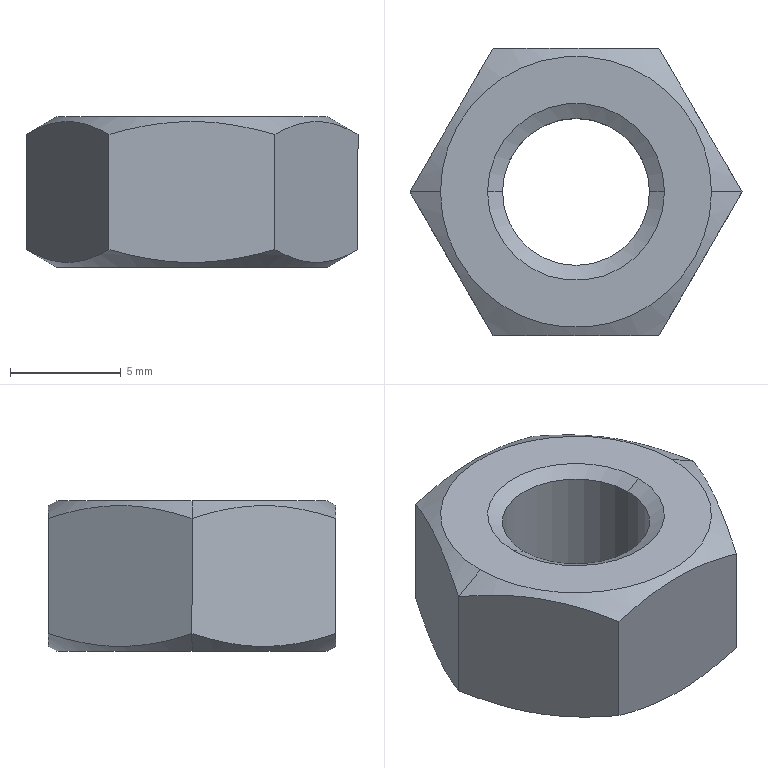Part | STEP file | hex nuts, style 1-grades ab gb_GB_FASTENER_NUT_SNAB1 M8-N | 1 solid | 18 faces | box 15.011 x 13 x 6.8 mm | volume 739.531 mm3 | cone 8 | plane 8 | cylinder 2 | commonest cylinder face diameters 6.647 x2
STEP:
#1=CARTESIAN_POINT('',(-3.324,0.,-0.3906));
#2=VERTEX_POINT('',#1);
#3=CARTESIAN_POINT('',(3.324,0.,-0.3906));
#4=VERTEX_POINT('',#3);
#5=CARTESIAN_POINT('',(0.,0.,-0.3906));
#6=DIRECTION('',(0.,0.,1.));
#7=DIRECTION('',(1.,0.,0.));
#8=AXIS2_PLACEMENT_3D('',#5,#6,#7);
#9=CIRCLE('',#8,3.324);
#10=EDGE_CURVE('',#2,#4,#9,.T.);
#11=ORIENTED_EDGE('',*,*,#10,.F.);
#12=CARTESIAN_POINT('',(-4.,0.,0.));
#13=VERTEX_POINT('',#12);
#14=CARTESIAN_POINT('',(-3.324,0.,-0.3906));
#15=DIRECTION('',(-0.866,0.,0.5));
#16=VECTOR('',#15,1000.);
#17=LINE('',#14,#16);
#18=EDGE_CURVE('',#2,#13,#17,.T.);
#19=ORIENTED_EDGE('',*,*,#18,.T.);
#20=CARTESIAN_POINT('',(4.,0.,0.));
#21=VERTEX_POINT('',#20);
#22=CARTESIAN_POINT('',(0.,0.,0.));
#23=DIRECTION('',(0.,0.,-1.));
#24=DIRECTION('',(1.,0.,0.));
#25=AXIS2_PLACEMENT_3D('',#22,#23,#24);
#26=CIRCLE('',#25,4.);
#27=EDGE_CURVE('',#21,#13,#26,.T.);
#28=ORIENTED_EDGE('',*,*,#27,.F.);
#29=CARTESIAN_POINT('',(3.324,0.,-0.3906));
#30=DIRECTION('',(0.866,0.,0.5));
#31=VECTOR('',#30,1000.);
#32=LINE('',#29,#31);
#33=EDGE_CURVE('',#4,#21,#32,.T.);
#34=ORIENTED_EDGE('',*,*,#33,.F.);
#35=EDGE_LOOP('',(#11,#19,#28,#34));
#36=FACE_OUTER_BOUND('',#35,.T.);
#37=CARTESIAN_POINT('',(0.,0.,-0.3906));
#38=DIRECTION('',(0.,0.,1.));
#39=DIRECTION('',(1.,0.,0.));
#40=AXIS2_PLACEMENT_3D('',#37,#38,#39);
#41=CONICAL_SURFACE('',#40,3.324,1.047);
#42=ADVANCED_FACE('',(#36),#41,.F.);
#43=CARTESIAN_POINT('',(3.324,0.,-6.124));
#44=VERTEX_POINT('',#43);
#45=CARTESIAN_POINT('',(-3.324,0.,-6.124));
#46=VERTEX_POINT('',#45);
#47=CARTESIAN_POINT('',(0.,0.,-6.124));
#48=DIRECTION('',(0.,0.,-1.));
#49=DIRECTION('',(1.,0.,0.));
#50=AXIS2_PLACEMENT_3D('',#47,#48,#49);
#51=CIRCLE('',#50,3.324);
#52=EDGE_CURVE('',#44,#46,#51,.T.);
#53=ORIENTED_EDGE('',*,*,#52,.F.);
#54=CARTESIAN_POINT('',(3.714,0.,-6.8));
#55=VERTEX_POINT('',#54);
#56=CARTESIAN_POINT('',(3.714,0.,-6.8));
#57=DIRECTION('',(0.5,0.,-0.866));
#58=VECTOR('',#57,1000.);
#59=LINE('',#56,#58);
#60=EDGE_CURVE('',#44,#55,#59,.T.);
#61=ORIENTED_EDGE('',*,*,#60,.T.);
#62=CARTESIAN_POINT('',(-3.714,0.,-6.8));
#63=VERTEX_POINT('',#62);
#64=CARTESIAN_POINT('',(0.,0.,-6.8));
#65=DIRECTION('',(0.,0.,1.));
#66=DIRECTION('',(1.,0.,0.));
#67=AXIS2_PLACEMENT_3D('',#64,#65,#66);
#68=CIRCLE('',#67,3.714);
#69=EDGE_CURVE('',#63,#55,#68,.T.);
#70=ORIENTED_EDGE('',*,*,#69,.F.);
#71=CARTESIAN_POINT('',(-3.714,0.,-6.8));
#72=DIRECTION('',(-0.5,0.,-0.866));
#73=VECTOR('',#72,1000.);
#74=LINE('',#71,#73);
#75=EDGE_CURVE('',#46,#63,#74,.T.);
#76=ORIENTED_EDGE('',*,*,#75,.F.);
#77=EDGE_LOOP('',(#53,#61,#70,#76));
#78=FACE_OUTER_BOUND('',#77,.T.);
#79=CARTESIAN_POINT('',(0.,0.,-6.8));
#80=DIRECTION('',(0.,0.,-1.));
#81=DIRECTION('',(-1.,0.,0.));
#82=AXIS2_PLACEMENT_3D('',#79,#80,#81);
#83=CONICAL_SURFACE('',#82,3.714,0.5236);
#84=ADVANCED_FACE('',(#78),#83,.F.);
#85=CARTESIAN_POINT('',(-6.125,0.,0.));
#86=VERTEX_POINT('',#85);
#87=CARTESIAN_POINT('',(6.125,0.,0.));
#88=VERTEX_POINT('',#87);
#89=CARTESIAN_POINT('',(0.,0.,0.));
#90=DIRECTION('',(0.,0.,-1.));
#91=DIRECTION('',(-1.,0.,0.));
#92=AXIS2_PLACEMENT_3D('',#89,#90,#91);
#93=CIRCLE('',#92,6.125);
#94=EDGE_CURVE('',#86,#88,#93,.T.);
#95=ORIENTED_EDGE('',*,*,#94,.T.);
#96=CARTESIAN_POINT('',(7.506,0.,-0.7971));
#97=VERTEX_POINT('',#96);
#98=CARTESIAN_POINT('',(6.125,0.,0.));
#99=DIRECTION('',(0.866,0.,-0.5));
#100=VECTOR('',#99,1000.);
#101=LINE('',#98,#100);
#102=EDGE_CURVE('',#88,#97,#101,.T.);
#103=ORIENTED_EDGE('',*,*,#102,.T.);
#104=CARTESIAN_POINT('',(3.753,6.5,-0.7971));
#105=VERTEX_POINT('',#104);
#106=CARTESIAN_POINT('',(7.506,0.,-0.7971));
#107=CARTESIAN_POINT('',(7.199,0.5307,-0.6202));
#108=CARTESIAN_POINT('',(6.891,1.065,-0.4744));
#109=CARTESIAN_POINT('',(6.267,2.145,-0.2724));
#110=CARTESIAN_POINT('',(5.952,2.691,-0.2169));
#111=CARTESIAN_POINT('',(5.473,3.52,-0.2163));
#112=CARTESIAN_POINT('',(5.313,3.798,-0.2299));
#113=CARTESIAN_POINT('',(4.996,4.347,-0.2828));
#114=CARTESIAN_POINT('',(4.838,4.62,-0.3221));
#115=CARTESIAN_POINT('',(4.369,5.433,-0.4738));
#116=CARTESIAN_POINT('',(4.06,5.969,-0.62));
#117=CARTESIAN_POINT('',(3.753,6.5,-0.7971));
#118=B_SPLINE_CURVE_WITH_KNOTS('',3,(#106,#107,#108,#109,#110,#111,#112,#113,#114,#115,#116,#117),.UNSPECIFIED.,.F.,.F.,(4,2,2,2,2,4),(0.000000238,0.001895,0.00379,0.004738,0.005685,0.00758),.UNSPECIFIED.);
#119=EDGE_CURVE('',#97,#105,#118,.T.);
#120=ORIENTED_EDGE('',*,*,#119,.T.);
#121=CARTESIAN_POINT('',(-3.753,6.5,-0.7971));
#122=VERTEX_POINT('',#121);
#123=CARTESIAN_POINT('',(3.753,6.5,-0.7971));
#124=CARTESIAN_POINT('',(3.146,6.5,-0.6219));
#125=CARTESIAN_POINT('',(2.532,6.5,-0.4761));
#126=CARTESIAN_POINT('',(1.278,6.5,-0.2726));
#127=CARTESIAN_POINT('',(0.6353,6.5,-0.2166));
#128=CARTESIAN_POINT('',(-0.6332,6.5,-0.2164));
#129=CARTESIAN_POINT('',(-1.263,6.5,-0.2709));
#130=CARTESIAN_POINT('',(-2.517,6.5,-0.473));
#131=CARTESIAN_POINT('',(-3.142,6.5,-0.6208));
#132=CARTESIAN_POINT('',(-3.753,6.5,-0.7971));
#133=B_SPLINE_CURVE_WITH_KNOTS('',3,(#123,#124,#125,#126,#127,#128,#129,#130,#131,#132),.UNSPECIFIED.,.F.,.F.,(4,2,2,2,4),(0.002787,0.004681,0.006575,0.008469,0.01036),.UNSPECIFIED.);
#134=EDGE_CURVE('',#105,#122,#133,.T.);
#135=ORIENTED_EDGE('',*,*,#134,.T.);
#136=CARTESIAN_POINT('',(-7.506,0.,-0.7971));
#137=VERTEX_POINT('',#136);
#138=CARTESIAN_POINT('',(-3.753,6.5,-0.7971));
#139=CARTESIAN_POINT('',(-4.059,5.969,-0.6202));
#140=CARTESIAN_POINT('',(-4.368,5.435,-0.4744));
#141=CARTESIAN_POINT('',(-4.991,4.355,-0.2724));
#142=CARTESIAN_POINT('',(-5.307,3.809,-0.2169));
#143=CARTESIAN_POINT('',(-5.785,2.98,-0.2163));
#144=CARTESIAN_POINT('',(-5.945,2.702,-0.2299));
#145=CARTESIAN_POINT('',(-6.262,2.153,-0.2828));
#146=CARTESIAN_POINT('',(-6.42,1.88,-0.3221));
#147=CARTESIAN_POINT('',(-6.889,1.067,-0.4738));
#148=CARTESIAN_POINT('',(-7.199,0.5313,-0.62));
#149=CARTESIAN_POINT('',(-7.506,0.,-0.7971));
#150=B_SPLINE_CURVE_WITH_KNOTS('',3,(#138,#139,#140,#141,#142,#143,#144,#145,#146,#147,#148,#149),.UNSPECIFIED.,.F.,.F.,(4,2,2,2,2,4),(0.000000238,0.001895,0.00379,0.004738,0.005685,0.00758),.UNSPECIFIED.);
#151=EDGE_CURVE('',#122,#137,#150,.T.);
#152=ORIENTED_EDGE('',*,*,#151,.T.);
#153=CARTESIAN_POINT('',(-6.125,0.,0.));
#154=DIRECTION('',(-0.866,0.,-0.5));
#155=VECTOR('',#154,1000.);
#156=LINE('',#153,#155);
#157=EDGE_CURVE('',#86,#137,#156,.T.);
#158=ORIENTED_EDGE('',*,*,#157,.F.);
#159=EDGE_LOOP('',(#95,#103,#120,#135,#152,#158));
#160=FACE_OUTER_BOUND('',#159,.T.);
#161=CARTESIAN_POINT('',(0.,0.,0.));
#162=DIRECTION('',(0.,0.,-1.));
#163=DIRECTION('',(-1.,0.,0.));
#164=AXIS2_PLACEMENT_3D('',#161,#162,#163);
#165=CONICAL_SURFACE('',#164,6.125,1.047);
#166=ADVANCED_FACE('',(#160),#165,.T.);
#167=CARTESIAN_POINT('',(-6.125,0.,-6.8));
#168=VERTEX_POINT('',#167);
#169=CARTESIAN_POINT('',(6.125,0.,-6.8));
#170=VERTEX_POINT('',#169);
#171=CARTESIAN_POINT('',(0.,0.,-6.8));
#172=DIRECTION('',(0.,0.,-1.));
#173=DIRECTION('',(-1.,0.,0.));
#174=AXIS2_PLACEMENT_3D('',#171,#172,#173);
#175=CIRCLE('',#174,6.125);
#176=EDGE_CURVE('',#168,#170,#175,.T.);
#177=ORIENTED_EDGE('',*,*,#176,.F.);
#178=CARTESIAN_POINT('',(-7.506,0.,-6.003));
#179=VERTEX_POINT('',#178);
#180=CARTESIAN_POINT('',(-7.506,0.,-6.003));
#181=DIRECTION('',(-0.866,0.,0.5));
#182=VECTOR('',#181,1000.);
#183=LINE('',#180,#182);
#184=EDGE_CURVE('',#168,#179,#183,.T.);
#185=ORIENTED_EDGE('',*,*,#184,.T.);
#186=CARTESIAN_POINT('',(-3.753,6.5,-6.003));
#187=VERTEX_POINT('',#186);
#188=CARTESIAN_POINT('',(-7.506,0.,-6.003));
#189=CARTESIAN_POINT('',(-7.199,0.5307,-6.18));
#190=CARTESIAN_POINT('',(-6.891,1.065,-6.326));
#191=CARTESIAN_POINT('',(-6.267,2.145,-6.528));
#192=CARTESIAN_POINT('',(-5.952,2.691,-6.583));
#193=CARTESIAN_POINT('',(-5.473,3.52,-6.584));
#194=CARTESIAN_POINT('',(-5.313,3.798,-6.57));
#195=CARTESIAN_POINT('',(-4.996,4.347,-6.517));
#196=CARTESIAN_POINT('',(-4.838,4.62,-6.478));
#197=CARTESIAN_POINT('',(-4.369,5.433,-6.326));
#198=CARTESIAN_POINT('',(-4.06,5.969,-6.18));
#199=CARTESIAN_POINT('',(-3.753,6.5,-6.003));
#200=B_SPLINE_CURVE_WITH_KNOTS('',3,(#188,#189,#190,#191,#192,#193,#194,#195,#196,#197,#198,#199),.UNSPECIFIED.,.F.,.F.,(4,2,2,2,2,4),(0.000000238,0.001895,0.00379,0.004738,0.005685,0.00758),.UNSPECIFIED.);
#201=EDGE_CURVE('',#179,#187,#200,.T.);
#202=ORIENTED_EDGE('',*,*,#201,.T.);
#203=CARTESIAN_POINT('',(3.753,6.5,-6.003));
#204=VERTEX_POINT('',#203);
#205=CARTESIAN_POINT('',(-3.753,6.5,-6.003));
#206=CARTESIAN_POINT('',(-3.142,6.5,-6.179));
#207=CARTESIAN_POINT('',(-2.517,6.5,-6.327));
#208=CARTESIAN_POINT('',(-1.263,6.5,-6.529));
#209=CARTESIAN_POINT('',(-0.6332,6.5,-6.584));
#210=CARTESIAN_POINT('',(0.6353,6.5,-6.583));
#211=CARTESIAN_POINT('',(1.278,6.5,-6.527));
#212=CARTESIAN_POINT('',(2.532,6.5,-6.324));
#213=CARTESIAN_POINT('',(3.146,6.5,-6.178));
#214=CARTESIAN_POINT('',(3.753,6.5,-6.003));
#215=B_SPLINE_CURVE_WITH_KNOTS('',3,(#205,#206,#207,#208,#209,#210,#211,#212,#213,#214),.UNSPECIFIED.,.F.,.F.,(4,2,2,2,4),(0.006662,0.008561,0.01046,0.01236,0.01426),.UNSPECIFIED.);
#216=EDGE_CURVE('',#187,#204,#215,.T.);
#217=ORIENTED_EDGE('',*,*,#216,.T.);
#218=CARTESIAN_POINT('',(7.506,0.,-6.003));
#219=VERTEX_POINT('',#218);
#220=CARTESIAN_POINT('',(3.753,6.5,-6.003));
#221=CARTESIAN_POINT('',(4.059,5.969,-6.18));
#222=CARTESIAN_POINT('',(4.368,5.435,-6.326));
#223=CARTESIAN_POINT('',(4.991,4.355,-6.528));
#224=CARTESIAN_POINT('',(5.307,3.809,-6.583));
#225=CARTESIAN_POINT('',(5.785,2.98,-6.584));
#226=CARTESIAN_POINT('',(5.945,2.702,-6.57));
#227=CARTESIAN_POINT('',(6.262,2.153,-6.517));
#228=CARTESIAN_POINT('',(6.42,1.88,-6.478));
#229=CARTESIAN_POINT('',(6.889,1.067,-6.326));
#230=CARTESIAN_POINT('',(7.199,0.5313,-6.18));
#231=CARTESIAN_POINT('',(7.506,0.,-6.003));
#232=B_SPLINE_CURVE_WITH_KNOTS('',3,(#220,#221,#222,#223,#224,#225,#226,#227,#228,#229,#230,#231),.UNSPECIFIED.,.F.,.F.,(4,2,2,2,2,4),(0.000000238,0.001895,0.00379,0.004738,0.005685,0.00758),.UNSPECIFIED.);
#233=EDGE_CURVE('',#204,#219,#232,.T.);
#234=ORIENTED_EDGE('',*,*,#233,.T.);
#235=CARTESIAN_POINT('',(7.506,0.,-6.003));
#236=DIRECTION('',(0.866,0.,0.5));
#237=VECTOR('',#236,1000.);
#238=LINE('',#235,#237);
#239=EDGE_CURVE('',#170,#219,#238,.T.);
#240=ORIENTED_EDGE('',*,*,#239,.F.);
#241=EDGE_LOOP('',(#177,#185,#202,#217,#234,#240));
#242=FACE_OUTER_BOUND('',#241,.T.);
#243=CARTESIAN_POINT('',(0.,0.,-6.003));
#244=DIRECTION('',(0.,0.,1.));
#245=DIRECTION('',(1.,0.,0.));
#246=AXIS2_PLACEMENT_3D('',#243,#244,#245);
#247=CONICAL_SURFACE('',#246,7.506,1.047);
#248=ADVANCED_FACE('',(#242),#247,.T.);
#249=ORIENTED_EDGE('',*,*,#52,.T.);
#250=CARTESIAN_POINT('',(-3.324,0.,-6.8));
#251=DIRECTION('',(0.,0.,1.));
#252=VECTOR('',#251,1000.);
#253=LINE('',#250,#252);
#254=EDGE_CURVE('',#46,#2,#253,.T.);
#255=ORIENTED_EDGE('',*,*,#254,.T.);
#256=ORIENTED_EDGE('',*,*,#10,.T.);
#257=CARTESIAN_POINT('',(3.324,0.,-6.8));
#258=DIRECTION('',(0.,0.,1.));
#259=VECTOR('',#258,1000.);
#260=LINE('',#257,#259);
#261=EDGE_CURVE('',#44,#4,#260,.T.);
#262=ORIENTED_EDGE('',*,*,#261,.F.);
#263=EDGE_LOOP('',(#249,#255,#256,#262));
#264=FACE_OUTER_BOUND('',#263,.T.);
#265=CARTESIAN_POINT('',(0.,0.,-6.8));
#266=DIRECTION('',(0.,0.,1.));
#267=DIRECTION('',(1.,0.,0.));
#268=AXIS2_PLACEMENT_3D('',#265,#266,#267);
#269=CYLINDRICAL_SURFACE('',#268,3.324);
#270=ADVANCED_FACE('',(#264),#269,.F.);
#271=CARTESIAN_POINT('',(3.753,-6.5,-0.7971));
#272=VERTEX_POINT('',#271);
#273=CARTESIAN_POINT('',(3.753,-6.5,-0.7971));
#274=CARTESIAN_POINT('',(4.059,-5.969,-0.6202));
#275=CARTESIAN_POINT('',(4.368,-5.435,-0.4744));
#276=CARTESIAN_POINT('',(4.991,-4.355,-0.2724));
#277=CARTESIAN_POINT('',(5.307,-3.809,-0.2169));
#278=CARTESIAN_POINT('',(5.785,-2.98,-0.2163));
#279=CARTESIAN_POINT('',(5.945,-2.702,-0.2299));
#280=CARTESIAN_POINT('',(6.262,-2.153,-0.2828));
#281=CARTESIAN_POINT('',(6.42,-1.88,-0.3221));
#282=CARTESIAN_POINT('',(6.889,-1.067,-0.4738));
#283=CARTESIAN_POINT('',(7.199,-0.5313,-0.62));
#284=CARTESIAN_POINT('',(7.506,0.,-0.7971));
#285=B_SPLINE_CURVE_WITH_KNOTS('',3,(#273,#274,#275,#276,#277,#278,#279,#280,#281,#282,#283,#284),.UNSPECIFIED.,.F.,.F.,(4,2,2,2,2,4),(0.000000238,0.001895,0.00379,0.004738,0.005685,0.00758),.UNSPECIFIED.);
#286=EDGE_CURVE('',#272,#97,#285,.T.);
#287=ORIENTED_EDGE('',*,*,#286,.F.);
#288=CARTESIAN_POINT('',(3.753,-6.5,-6.003));
#289=VERTEX_POINT('',#288);
#290=CARTESIAN_POINT('',(3.753,-6.5,-6.8));
#291=DIRECTION('',(0.,0.,1.));
#292=VECTOR('',#291,1000.);
#293=LINE('',#290,#292);
#294=EDGE_CURVE('',#289,#272,#293,.T.);
#295=ORIENTED_EDGE('',*,*,#294,.F.);
#296=CARTESIAN_POINT('',(7.506,0.,-6.003));
#297=CARTESIAN_POINT('',(7.199,-0.5307,-6.18));
#298=CARTESIAN_POINT('',(6.891,-1.065,-6.326));
#299=CARTESIAN_POINT('',(6.267,-2.145,-6.528));
#300=CARTESIAN_POINT('',(5.952,-2.691,-6.583));
#301=CARTESIAN_POINT('',(5.473,-3.52,-6.584));
#302=CARTESIAN_POINT('',(5.313,-3.798,-6.57));
#303=CARTESIAN_POINT('',(4.996,-4.347,-6.517));
#304=CARTESIAN_POINT('',(4.838,-4.62,-6.478));
#305=CARTESIAN_POINT('',(4.369,-5.433,-6.326));
#306=CARTESIAN_POINT('',(4.06,-5.969,-6.18));
#307=CARTESIAN_POINT('',(3.753,-6.5,-6.003));
#308=B_SPLINE_CURVE_WITH_KNOTS('',3,(#296,#297,#298,#299,#300,#301,#302,#303,#304,#305,#306,#307),.UNSPECIFIED.,.F.,.F.,(4,2,2,2,2,4),(0.000000238,0.001895,0.00379,0.004738,0.005685,0.00758),.UNSPECIFIED.);
#309=EDGE_CURVE('',#219,#289,#308,.T.);
#310=ORIENTED_EDGE('',*,*,#309,.F.);
#311=CARTESIAN_POINT('',(7.506,0.,-6.8));
#312=DIRECTION('',(0.,0.,1.));
#313=VECTOR('',#312,1000.);
#314=LINE('',#311,#313);
#315=EDGE_CURVE('',#219,#97,#314,.T.);
#316=ORIENTED_EDGE('',*,*,#315,.T.);
#317=EDGE_LOOP('',(#287,#295,#310,#316));
#318=FACE_OUTER_BOUND('',#317,.T.);
#319=CARTESIAN_POINT('',(3.753,-6.5,-6.8));
#320=DIRECTION('',(0.866,-0.5,0.));
#321=DIRECTION('',(0.5,0.866,0.));
#322=AXIS2_PLACEMENT_3D('',#319,#320,#321);
#323=PLANE('',#322);
#324=ADVANCED_FACE('',(#318),#323,.T.);
#325=CARTESIAN_POINT('',(-3.753,-6.5,-0.7971));
#326=VERTEX_POINT('',#325);
#327=CARTESIAN_POINT('',(-3.753,-6.5,-0.7971));
#328=CARTESIAN_POINT('',(-3.142,-6.5,-0.6208));
#329=CARTESIAN_POINT('',(-2.517,-6.5,-0.473));
#330=CARTESIAN_POINT('',(-1.263,-6.5,-0.2709));
#331=CARTESIAN_POINT('',(-0.6332,-6.5,-0.2164));
#332=CARTESIAN_POINT('',(0.6353,-6.5,-0.2166));
#333=CARTESIAN_POINT('',(1.278,-6.5,-0.2726));
#334=CARTESIAN_POINT('',(2.532,-6.5,-0.4761));
#335=CARTESIAN_POINT('',(3.146,-6.5,-0.6219));
#336=CARTESIAN_POINT('',(3.753,-6.5,-0.7971));
#337=B_SPLINE_CURVE_WITH_KNOTS('',3,(#327,#328,#329,#330,#331,#332,#333,#334,#335,#336),.UNSPECIFIED.,.F.,.F.,(4,2,2,2,4),(0.006662,0.008561,0.01046,0.01236,0.01426),.UNSPECIFIED.);
#338=EDGE_CURVE('',#326,#272,#337,.T.);
#339=ORIENTED_EDGE('',*,*,#338,.F.);
#340=CARTESIAN_POINT('',(-3.753,-6.5,-6.003));
#341=VERTEX_POINT('',#340);
#342=CARTESIAN_POINT('',(-3.753,-6.5,-6.8));
#343=DIRECTION('',(0.,0.,1.));
#344=VECTOR('',#343,1000.);
#345=LINE('',#342,#344);
#346=EDGE_CURVE('',#341,#326,#345,.T.);
#347=ORIENTED_EDGE('',*,*,#346,.F.);
#348=CARTESIAN_POINT('',(3.753,-6.5,-6.003));
#349=CARTESIAN_POINT('',(3.146,-6.5,-6.178));
#350=CARTESIAN_POINT('',(2.532,-6.5,-6.324));
#351=CARTESIAN_POINT('',(1.278,-6.5,-6.527));
#352=CARTESIAN_POINT('',(0.6353,-6.5,-6.583));
#353=CARTESIAN_POINT('',(-0.6332,-6.5,-6.584));
#354=CARTESIAN_POINT('',(-1.263,-6.5,-6.529));
#355=CARTESIAN_POINT('',(-2.517,-6.5,-6.327));
#356=CARTESIAN_POINT('',(-3.142,-6.5,-6.179));
#357=CARTESIAN_POINT('',(-3.753,-6.5,-6.003));
#358=B_SPLINE_CURVE_WITH_KNOTS('',3,(#348,#349,#350,#351,#352,#353,#354,#355,#356,#357),.UNSPECIFIED.,.F.,.F.,(4,2,2,2,4),(0.002787,0.004681,0.006575,0.008469,0.01036),.UNSPECIFIED.);
#359=EDGE_CURVE('',#289,#341,#358,.T.);
#360=ORIENTED_EDGE('',*,*,#359,.F.);
#361=ORIENTED_EDGE('',*,*,#294,.T.);
#362=EDGE_LOOP('',(#339,#347,#360,#361));
#363=FACE_OUTER_BOUND('',#362,.T.);
#364=CARTESIAN_POINT('',(-3.753,-6.5,-6.8));
#365=DIRECTION('',(0.,-1.,0.));
#366=DIRECTION('',(0.,0.,-1.));
#367=AXIS2_PLACEMENT_3D('',#364,#365,#366);
#368=PLANE('',#367);
#369=ADVANCED_FACE('',(#363),#368,.T.);
#370=CARTESIAN_POINT('',(-7.506,0.,-0.7971));
#371=CARTESIAN_POINT('',(-7.199,-0.5307,-0.6202));
#372=CARTESIAN_POINT('',(-6.891,-1.065,-0.4744));
#373=CARTESIAN_POINT('',(-6.267,-2.145,-0.2724));
#374=CARTESIAN_POINT('',(-5.952,-2.691,-0.2169));
#375=CARTESIAN_POINT('',(-5.473,-3.52,-0.2163));
#376=CARTESIAN_POINT('',(-5.313,-3.798,-0.2299));
#377=CARTESIAN_POINT('',(-4.996,-4.347,-0.2828));
#378=CARTESIAN_POINT('',(-4.838,-4.62,-0.3221));
#379=CARTESIAN_POINT('',(-4.369,-5.433,-0.4738));
#380=CARTESIAN_POINT('',(-4.06,-5.969,-0.62));
#381=CARTESIAN_POINT('',(-3.753,-6.5,-0.7971));
#382=B_SPLINE_CURVE_WITH_KNOTS('',3,(#370,#371,#372,#373,#374,#375,#376,#377,#378,#379,#380,#381),.UNSPECIFIED.,.F.,.F.,(4,2,2,2,2,4),(0.000000238,0.001895,0.00379,0.004738,0.005685,0.00758),.UNSPECIFIED.);
#383=EDGE_CURVE('',#137,#326,#382,.T.);
#384=ORIENTED_EDGE('',*,*,#383,.F.);
#385=CARTESIAN_POINT('',(-7.506,0.,-6.8));
#386=DIRECTION('',(0.,0.,1.));
#387=VECTOR('',#386,1000.);
#388=LINE('',#385,#387);
#389=EDGE_CURVE('',#179,#137,#388,.T.);
#390=ORIENTED_EDGE('',*,*,#389,.F.);
#391=CARTESIAN_POINT('',(-3.753,-6.5,-6.003));
#392=CARTESIAN_POINT('',(-4.059,-5.969,-6.18));
#393=CARTESIAN_POINT('',(-4.368,-5.435,-6.326));
#394=CARTESIAN_POINT('',(-4.991,-4.355,-6.528));
#395=CARTESIAN_POINT('',(-5.307,-3.809,-6.583));
#396=CARTESIAN_POINT('',(-5.785,-2.98,-6.584));
#397=CARTESIAN_POINT('',(-5.945,-2.702,-6.57));
#398=CARTESIAN_POINT('',(-6.262,-2.153,-6.517));
#399=CARTESIAN_POINT('',(-6.42,-1.88,-6.478));
#400=CARTESIAN_POINT('',(-6.889,-1.067,-6.326));
#401=CARTESIAN_POINT('',(-7.199,-0.5313,-6.18));
#402=CARTESIAN_POINT('',(-7.506,0.,-6.003));
#403=B_SPLINE_CURVE_WITH_KNOTS('',3,(#391,#392,#393,#394,#395,#396,#397,#398,#399,#400,#401,#402),.UNSPECIFIED.,.F.,.F.,(4,2,2,2,2,4),(0.000000238,0.001895,0.00379,0.004738,0.005685,0.00758),.UNSPECIFIED.);
#404=EDGE_CURVE('',#341,#179,#403,.T.);
#405=ORIENTED_EDGE('',*,*,#404,.F.);
#406=ORIENTED_EDGE('',*,*,#346,.T.);
#407=EDGE_LOOP('',(#384,#390,#405,#406));
#408=FACE_OUTER_BOUND('',#407,.T.);
#409=CARTESIAN_POINT('',(-7.506,0.,-6.8));
#410=DIRECTION('',(-0.866,-0.5,0.));
#411=DIRECTION('',(0.5,-0.866,0.));
#412=AXIS2_PLACEMENT_3D('',#409,#410,#411);
#413=PLANE('',#412);
#414=ADVANCED_FACE('',(#408),#413,.T.);
#415=ORIENTED_EDGE('',*,*,#151,.F.);
#416=CARTESIAN_POINT('',(-3.753,6.5,-6.8));
#417=DIRECTION('',(0.,0.,1.));
#418=VECTOR('',#417,1000.);
#419=LINE('',#416,#418);
#420=EDGE_CURVE('',#187,#122,#419,.T.);
#421=ORIENTED_EDGE('',*,*,#420,.F.);
#422=ORIENTED_EDGE('',*,*,#201,.F.);
#423=ORIENTED_EDGE('',*,*,#389,.T.);
#424=EDGE_LOOP('',(#415,#421,#422,#423));
#425=FACE_OUTER_BOUND('',#424,.T.);
#426=CARTESIAN_POINT('',(-3.753,6.5,-6.8));
#427=DIRECTION('',(-0.866,0.5,0.));
#428=DIRECTION('',(-0.5,-0.866,0.));
#429=AXIS2_PLACEMENT_3D('',#426,#427,#428);
#430=PLANE('',#429);
#431=ADVANCED_FACE('',(#425),#430,.T.);
#432=ORIENTED_EDGE('',*,*,#134,.F.);
#433=CARTESIAN_POINT('',(3.753,6.5,-6.8));
#434=DIRECTION('',(0.,0.,1.));
#435=VECTOR('',#434,1000.);
#436=LINE('',#433,#435);
#437=EDGE_CURVE('',#204,#105,#436,.T.);
#438=ORIENTED_EDGE('',*,*,#437,.F.);
#439=ORIENTED_EDGE('',*,*,#216,.F.);
#440=ORIENTED_EDGE('',*,*,#420,.T.);
#441=EDGE_LOOP('',(#432,#438,#439,#440));
#442=FACE_OUTER_BOUND('',#441,.T.);
#443=CARTESIAN_POINT('',(3.753,6.5,-6.8));
#444=DIRECTION('',(0.,1.,0.));
#445=DIRECTION('',(0.,0.,1.));
#446=AXIS2_PLACEMENT_3D('',#443,#444,#445);
#447=PLANE('',#446);
#448=ADVANCED_FACE('',(#442),#447,.T.);
#449=ORIENTED_EDGE('',*,*,#119,.F.);
#450=ORIENTED_EDGE('',*,*,#315,.F.);
#451=ORIENTED_EDGE('',*,*,#233,.F.);
#452=ORIENTED_EDGE('',*,*,#437,.T.);
#453=EDGE_LOOP('',(#449,#450,#451,#452));
#454=FACE_OUTER_BOUND('',#453,.T.);
#455=CARTESIAN_POINT('',(7.506,0.,-6.8));
#456=DIRECTION('',(0.866,0.5,0.));
#457=DIRECTION('',(-0.5,0.866,0.));
#458=AXIS2_PLACEMENT_3D('',#455,#456,#457);
#459=PLANE('',#458);
#460=ADVANCED_FACE('',(#454),#459,.T.);
#461=ORIENTED_EDGE('',*,*,#69,.T.);
#462=CARTESIAN_POINT('',(0.,0.,-6.8));
#463=DIRECTION('',(0.,0.,1.));
#464=DIRECTION('',(1.,0.,0.));
#465=AXIS2_PLACEMENT_3D('',#462,#463,#464);
#466=CIRCLE('',#465,3.714);
#467=EDGE_CURVE('',#55,#63,#466,.T.);
#468=ORIENTED_EDGE('',*,*,#467,.T.);
#469=EDGE_LOOP('',(#461,#468));
#470=FACE_BOUND('',#469,.T.);
#471=CARTESIAN_POINT('',(0.,0.,-6.8));
#472=DIRECTION('',(0.,0.,-1.));
#473=DIRECTION('',(-1.,0.,0.));
#474=AXIS2_PLACEMENT_3D('',#471,#472,#473);
#475=CIRCLE('',#474,6.125);
#476=EDGE_CURVE('',#170,#168,#475,.T.);
#477=ORIENTED_EDGE('',*,*,#476,.T.);
#478=ORIENTED_EDGE('',*,*,#176,.T.);
#479=EDGE_LOOP('',(#477,#478));
#480=FACE_OUTER_BOUND('',#479,.T.);
#481=CARTESIAN_POINT('',(7.506,0.,-6.8));
#482=DIRECTION('',(0.,0.,1.));
#483=DIRECTION('',(1.,0.,0.));
#484=AXIS2_PLACEMENT_3D('',#481,#482,#483);
#485=PLANE('',#484);
#486=ADVANCED_FACE('',(#470,#480),#485,.F.);
#487=ORIENTED_EDGE('',*,*,#27,.T.);
#488=CARTESIAN_POINT('',(0.,0.,0.));
#489=DIRECTION('',(0.,0.,-1.));
#490=DIRECTION('',(1.,0.,0.));
#491=AXIS2_PLACEMENT_3D('',#488,#489,#490);
#492=CIRCLE('',#491,4.);
#493=EDGE_CURVE('',#13,#21,#492,.T.);
#494=ORIENTED_EDGE('',*,*,#493,.T.);
#495=EDGE_LOOP('',(#487,#494));
#496=FACE_BOUND('',#495,.T.);
#497=ORIENTED_EDGE('',*,*,#94,.F.);
#498=CARTESIAN_POINT('',(0.,0.,0.));
#499=DIRECTION('',(0.,0.,-1.));
#500=DIRECTION('',(-1.,0.,0.));
#501=AXIS2_PLACEMENT_3D('',#498,#499,#500);
#502=CIRCLE('',#501,6.125);
#503=EDGE_CURVE('',#88,#86,#502,.T.);
#504=ORIENTED_EDGE('',*,*,#503,.F.);
#505=EDGE_LOOP('',(#497,#504));
#506=FACE_OUTER_BOUND('',#505,.T.);
#507=CARTESIAN_POINT('',(7.506,0.,0.));
#508=DIRECTION('',(0.,0.,1.));
#509=DIRECTION('',(1.,0.,0.));
#510=AXIS2_PLACEMENT_3D('',#507,#508,#509);
#511=PLANE('',#510);
#512=ADVANCED_FACE('',(#496,#506),#511,.T.);
#513=ORIENTED_EDGE('',*,*,#254,.F.);
#514=CARTESIAN_POINT('',(0.,0.,-6.124));
#515=DIRECTION('',(0.,0.,-1.));
#516=DIRECTION('',(1.,0.,0.));
#517=AXIS2_PLACEMENT_3D('',#514,#515,#516);
#518=CIRCLE('',#517,3.324);
#519=EDGE_CURVE('',#46,#44,#518,.T.);
#520=ORIENTED_EDGE('',*,*,#519,.T.);
#521=ORIENTED_EDGE('',*,*,#261,.T.);
#522=CARTESIAN_POINT('',(0.,0.,-0.3906));
#523=DIRECTION('',(0.,0.,1.));
#524=DIRECTION('',(1.,0.,0.));
#525=AXIS2_PLACEMENT_3D('',#522,#523,#524);
#526=CIRCLE('',#525,3.324);
#527=EDGE_CURVE('',#4,#2,#526,.T.);
#528=ORIENTED_EDGE('',*,*,#527,.T.);
#529=EDGE_LOOP('',(#513,#520,#521,#528));
#530=FACE_OUTER_BOUND('',#529,.T.);
#531=CARTESIAN_POINT('',(0.,0.,-6.8));
#532=DIRECTION('',(0.,0.,1.));
#533=DIRECTION('',(1.,0.,0.));
#534=AXIS2_PLACEMENT_3D('',#531,#532,#533);
#535=CYLINDRICAL_SURFACE('',#534,3.324);
#536=ADVANCED_FACE('',(#530),#535,.F.);
#537=ORIENTED_EDGE('',*,*,#184,.F.);
#538=ORIENTED_EDGE('',*,*,#476,.F.);
#539=ORIENTED_EDGE('',*,*,#239,.T.);
#540=ORIENTED_EDGE('',*,*,#309,.T.);
#541=ORIENTED_EDGE('',*,*,#359,.T.);
#542=ORIENTED_EDGE('',*,*,#404,.T.);
#543=EDGE_LOOP('',(#537,#538,#539,#540,#541,#542));
#544=FACE_OUTER_BOUND('',#543,.T.);
#545=CARTESIAN_POINT('',(0.,0.,-6.003));
#546=DIRECTION('',(0.,0.,1.));
#547=DIRECTION('',(1.,0.,0.));
#548=AXIS2_PLACEMENT_3D('',#545,#546,#547);
#549=CONICAL_SURFACE('',#548,7.506,1.047);
#550=ADVANCED_FACE('',(#544),#549,.T.);
#551=ORIENTED_EDGE('',*,*,#102,.F.);
#552=ORIENTED_EDGE('',*,*,#503,.T.);
#553=ORIENTED_EDGE('',*,*,#157,.T.);
#554=ORIENTED_EDGE('',*,*,#383,.T.);
#555=ORIENTED_EDGE('',*,*,#338,.T.);
#556=ORIENTED_EDGE('',*,*,#286,.T.);
#557=EDGE_LOOP('',(#551,#552,#553,#554,#555,#556));
#558=FACE_OUTER_BOUND('',#557,.T.);
#559=CARTESIAN_POINT('',(0.,0.,0.));
#560=DIRECTION('',(0.,0.,-1.));
#561=DIRECTION('',(-1.,0.,0.));
#562=AXIS2_PLACEMENT_3D('',#559,#560,#561);
#563=CONICAL_SURFACE('',#562,6.125,1.047);
#564=ADVANCED_FACE('',(#558),#563,.T.);
#565=ORIENTED_EDGE('',*,*,#60,.F.);
#566=ORIENTED_EDGE('',*,*,#519,.F.);
#567=ORIENTED_EDGE('',*,*,#75,.T.);
#568=ORIENTED_EDGE('',*,*,#467,.F.);
#569=EDGE_LOOP('',(#565,#566,#567,#568));
#570=FACE_OUTER_BOUND('',#569,.T.);
#571=CARTESIAN_POINT('',(0.,0.,-6.8));
#572=DIRECTION('',(0.,0.,-1.));
#573=DIRECTION('',(-1.,0.,0.));
#574=AXIS2_PLACEMENT_3D('',#571,#572,#573);
#575=CONICAL_SURFACE('',#574,3.714,0.5236);
#576=ADVANCED_FACE('',(#570),#575,.F.);
#577=ORIENTED_EDGE('',*,*,#18,.F.);
#578=ORIENTED_EDGE('',*,*,#527,.F.);
#579=ORIENTED_EDGE('',*,*,#33,.T.);
#580=ORIENTED_EDGE('',*,*,#493,.F.);
#581=EDGE_LOOP('',(#577,#578,#579,#580));
#582=FACE_OUTER_BOUND('',#581,.T.);
#583=CARTESIAN_POINT('',(0.,0.,-0.3906));
#584=DIRECTION('',(0.,0.,1.));
#585=DIRECTION('',(1.,0.,0.));
#586=AXIS2_PLACEMENT_3D('',#583,#584,#585);
#587=CONICAL_SURFACE('',#586,3.324,1.047);
#588=ADVANCED_FACE('',(#582),#587,.F.);
#589=CLOSED_SHELL('',(#42,#84,#166,#248,#270,#324,#369,#414,#431,#448,#460,#486,#512,#536,#550,#564,#576,#588));
#590=MANIFOLD_SOLID_BREP('',#589);
#591=CARTESIAN_POINT('',(0.,0.,0.));
#592=DIRECTION('',(0.,0.,1.));
#593=DIRECTION('',(1.,0.,0.));
#594=AXIS2_PLACEMENT_3D('',#591,#592,#593);
#595=(LENGTH_UNIT()NAMED_UNIT(*)SI_UNIT(.MILLI.,.METRE.));
#596=UNCERTAINTY_MEASURE_WITH_UNIT(LENGTH_MEASURE(0.00001),#595,'','');
#597=(NAMED_UNIT(*)PLANE_ANGLE_UNIT()SI_UNIT($,.RADIAN.));
#598=(NAMED_UNIT(*)SI_UNIT($,.STERADIAN.)SOLID_ANGLE_UNIT());
#599=(GEOMETRIC_REPRESENTATION_CONTEXT(3)GLOBAL_UNCERTAINTY_ASSIGNED_CONTEXT((#596))GLOBAL_UNIT_ASSIGNED_CONTEXT((#595,#597,#598))REPRESENTATION_CONTEXT('',''));
#600=ADVANCED_BREP_SHAPE_REPRESENTATION('',(#590,#594),#599);